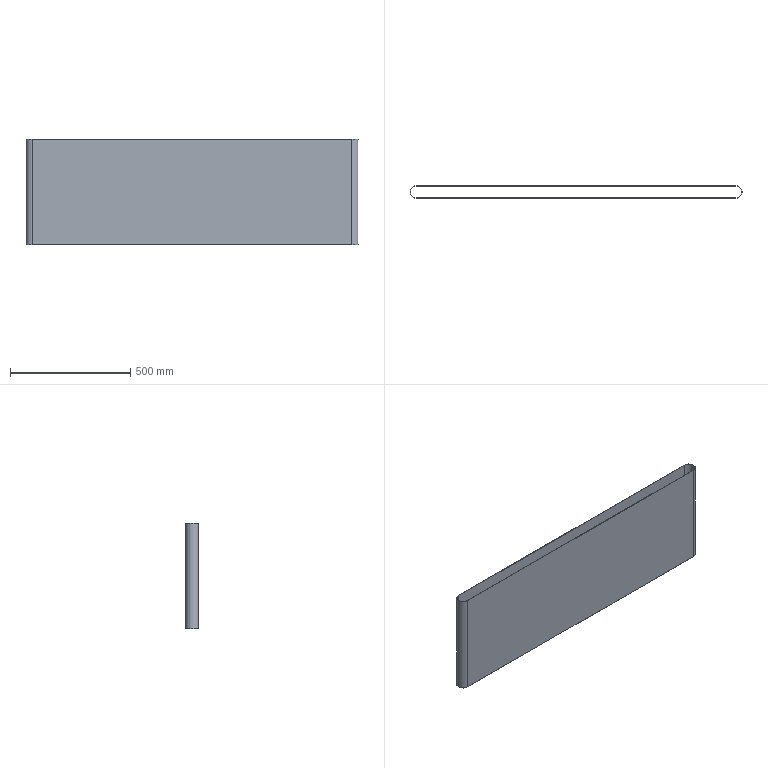Part | STEP file | RUBE 615 | 1 solid | 10 faces | box 1381 x 53.2 x 440 mm | volume 1983947 mm3 | plane 6 | cylinder 4 | commonest cylinder face diameters 50 x2 53.2 x2
STEP:
#1=CARTESIAN_POINT('',(-1248.5,28.6,220.));
#2=VERTEX_POINT('',#1);
#3=CARTESIAN_POINT('',(-1248.5,-24.6,220.));
#4=VERTEX_POINT('',#3);
#5=CARTESIAN_POINT('',(-1248.5,2.,220.));
#6=DIRECTION('',(0.,0.,1.));
#7=DIRECTION('',(1.,0.,0.));
#8=AXIS2_PLACEMENT_3D('',#5,#6,#7);
#9=CIRCLE('',#8,26.6);
#10=EDGE_CURVE('',#2,#4,#9,.T.);
#11=ORIENTED_EDGE('',*,*,#10,.T.);
#12=CARTESIAN_POINT('',(79.5,-24.6,220.));
#13=VERTEX_POINT('',#12);
#14=CARTESIAN_POINT('',(-1248.5,-24.6,220.));
#15=DIRECTION('',(1.,0.,0.));
#16=VECTOR('',#15,1000.);
#17=LINE('',#14,#16);
#18=EDGE_CURVE('',#4,#13,#17,.T.);
#19=ORIENTED_EDGE('',*,*,#18,.T.);
#20=CARTESIAN_POINT('',(79.5,28.6,220.));
#21=VERTEX_POINT('',#20);
#22=CARTESIAN_POINT('',(79.5,2.,220.));
#23=DIRECTION('',(0.,0.,1.));
#24=DIRECTION('',(1.,0.,0.));
#25=AXIS2_PLACEMENT_3D('',#22,#23,#24);
#26=CIRCLE('',#25,26.6);
#27=EDGE_CURVE('',#13,#21,#26,.T.);
#28=ORIENTED_EDGE('',*,*,#27,.T.);
#29=CARTESIAN_POINT('',(-1248.5,28.6,220.));
#30=DIRECTION('',(-1.,0.,0.));
#31=VECTOR('',#30,1000.);
#32=LINE('',#29,#31);
#33=EDGE_CURVE('',#21,#2,#32,.T.);
#34=ORIENTED_EDGE('',*,*,#33,.T.);
#35=EDGE_LOOP('',(#11,#19,#28,#34));
#36=FACE_OUTER_BOUND('',#35,.T.);
#37=CARTESIAN_POINT('',(-1248.5,-23.,220.));
#38=VERTEX_POINT('',#37);
#39=CARTESIAN_POINT('',(79.5,-23.,220.));
#40=VERTEX_POINT('',#39);
#41=CARTESIAN_POINT('',(-1248.5,-23.,220.));
#42=DIRECTION('',(1.,0.,0.));
#43=VECTOR('',#42,1000.);
#44=LINE('',#41,#43);
#45=EDGE_CURVE('',#38,#40,#44,.T.);
#46=ORIENTED_EDGE('',*,*,#45,.F.);
#47=CARTESIAN_POINT('',(-1248.5,27.,220.));
#48=VERTEX_POINT('',#47);
#49=CARTESIAN_POINT('',(-1248.5,2.,220.));
#50=DIRECTION('',(0.,0.,1.));
#51=DIRECTION('',(1.,0.,0.));
#52=AXIS2_PLACEMENT_3D('',#49,#50,#51);
#53=CIRCLE('',#52,25.);
#54=EDGE_CURVE('',#48,#38,#53,.T.);
#55=ORIENTED_EDGE('',*,*,#54,.F.);
#56=CARTESIAN_POINT('',(79.5,27.,220.));
#57=VERTEX_POINT('',#56);
#58=CARTESIAN_POINT('',(-1248.5,27.,220.));
#59=DIRECTION('',(-1.,0.,0.));
#60=VECTOR('',#59,1000.);
#61=LINE('',#58,#60);
#62=EDGE_CURVE('',#57,#48,#61,.T.);
#63=ORIENTED_EDGE('',*,*,#62,.F.);
#64=CARTESIAN_POINT('',(79.5,2.,220.));
#65=DIRECTION('',(0.,0.,1.));
#66=DIRECTION('',(1.,0.,0.));
#67=AXIS2_PLACEMENT_3D('',#64,#65,#66);
#68=CIRCLE('',#67,25.);
#69=EDGE_CURVE('',#40,#57,#68,.T.);
#70=ORIENTED_EDGE('',*,*,#69,.F.);
#71=EDGE_LOOP('',(#46,#55,#63,#70));
#72=FACE_BOUND('',#71,.T.);
#73=CARTESIAN_POINT('',(-1248.5,2.,220.));
#74=DIRECTION('',(0.,0.,1.));
#75=DIRECTION('',(1.,0.,0.));
#76=AXIS2_PLACEMENT_3D('',#73,#74,#75);
#77=PLANE('',#76);
#78=ADVANCED_FACE('',(#36,#72),#77,.T.);
#79=CARTESIAN_POINT('',(-1248.5,28.6,-220.));
#80=VERTEX_POINT('',#79);
#81=CARTESIAN_POINT('',(-1248.5,-24.6,-220.));
#82=VERTEX_POINT('',#81);
#83=CARTESIAN_POINT('',(-1248.5,2.,-220.));
#84=DIRECTION('',(0.,0.,1.));
#85=DIRECTION('',(1.,0.,0.));
#86=AXIS2_PLACEMENT_3D('',#83,#84,#85);
#87=CIRCLE('',#86,26.6);
#88=EDGE_CURVE('',#80,#82,#87,.T.);
#89=ORIENTED_EDGE('',*,*,#88,.F.);
#90=CARTESIAN_POINT('',(79.5,28.6,-220.));
#91=VERTEX_POINT('',#90);
#92=CARTESIAN_POINT('',(-1248.5,28.6,-220.));
#93=DIRECTION('',(-1.,0.,0.));
#94=VECTOR('',#93,1000.);
#95=LINE('',#92,#94);
#96=EDGE_CURVE('',#91,#80,#95,.T.);
#97=ORIENTED_EDGE('',*,*,#96,.F.);
#98=CARTESIAN_POINT('',(79.5,-24.6,-220.));
#99=VERTEX_POINT('',#98);
#100=CARTESIAN_POINT('',(79.5,2.,-220.));
#101=DIRECTION('',(0.,0.,1.));
#102=DIRECTION('',(1.,0.,0.));
#103=AXIS2_PLACEMENT_3D('',#100,#101,#102);
#104=CIRCLE('',#103,26.6);
#105=EDGE_CURVE('',#99,#91,#104,.T.);
#106=ORIENTED_EDGE('',*,*,#105,.F.);
#107=CARTESIAN_POINT('',(-1248.5,-24.6,-220.));
#108=DIRECTION('',(1.,0.,0.));
#109=VECTOR('',#108,1000.);
#110=LINE('',#107,#109);
#111=EDGE_CURVE('',#82,#99,#110,.T.);
#112=ORIENTED_EDGE('',*,*,#111,.F.);
#113=EDGE_LOOP('',(#89,#97,#106,#112));
#114=FACE_OUTER_BOUND('',#113,.T.);
#115=CARTESIAN_POINT('',(-1248.5,27.,-220.));
#116=VERTEX_POINT('',#115);
#117=CARTESIAN_POINT('',(-1248.5,-23.,-220.));
#118=VERTEX_POINT('',#117);
#119=CARTESIAN_POINT('',(-1248.5,2.,-220.));
#120=DIRECTION('',(0.,0.,1.));
#121=DIRECTION('',(1.,0.,0.));
#122=AXIS2_PLACEMENT_3D('',#119,#120,#121);
#123=CIRCLE('',#122,25.);
#124=EDGE_CURVE('',#116,#118,#123,.T.);
#125=ORIENTED_EDGE('',*,*,#124,.T.);
#126=CARTESIAN_POINT('',(79.5,-23.,-220.));
#127=VERTEX_POINT('',#126);
#128=CARTESIAN_POINT('',(-1248.5,-23.,-220.));
#129=DIRECTION('',(1.,0.,0.));
#130=VECTOR('',#129,1000.);
#131=LINE('',#128,#130);
#132=EDGE_CURVE('',#118,#127,#131,.T.);
#133=ORIENTED_EDGE('',*,*,#132,.T.);
#134=CARTESIAN_POINT('',(79.5,27.,-220.));
#135=VERTEX_POINT('',#134);
#136=CARTESIAN_POINT('',(79.5,2.,-220.));
#137=DIRECTION('',(0.,0.,1.));
#138=DIRECTION('',(1.,0.,0.));
#139=AXIS2_PLACEMENT_3D('',#136,#137,#138);
#140=CIRCLE('',#139,25.);
#141=EDGE_CURVE('',#127,#135,#140,.T.);
#142=ORIENTED_EDGE('',*,*,#141,.T.);
#143=CARTESIAN_POINT('',(-1248.5,27.,-220.));
#144=DIRECTION('',(-1.,0.,0.));
#145=VECTOR('',#144,1000.);
#146=LINE('',#143,#145);
#147=EDGE_CURVE('',#135,#116,#146,.T.);
#148=ORIENTED_EDGE('',*,*,#147,.T.);
#149=EDGE_LOOP('',(#125,#133,#142,#148));
#150=FACE_BOUND('',#149,.T.);
#151=CARTESIAN_POINT('',(-1248.5,2.,-220.));
#152=DIRECTION('',(0.,0.,1.));
#153=DIRECTION('',(1.,0.,0.));
#154=AXIS2_PLACEMENT_3D('',#151,#152,#153);
#155=PLANE('',#154);
#156=ADVANCED_FACE('',(#114,#150),#155,.F.);
#157=ORIENTED_EDGE('',*,*,#88,.T.);
#158=CARTESIAN_POINT('',(-1248.5,-24.6,220.));
#159=DIRECTION('',(0.,0.,-1.));
#160=VECTOR('',#159,1000.);
#161=LINE('',#158,#160);
#162=EDGE_CURVE('',#4,#82,#161,.T.);
#163=ORIENTED_EDGE('',*,*,#162,.F.);
#164=ORIENTED_EDGE('',*,*,#10,.F.);
#165=CARTESIAN_POINT('',(-1248.5,28.6,220.));
#166=DIRECTION('',(0.,0.,-1.));
#167=VECTOR('',#166,1000.);
#168=LINE('',#165,#167);
#169=EDGE_CURVE('',#2,#80,#168,.T.);
#170=ORIENTED_EDGE('',*,*,#169,.T.);
#171=EDGE_LOOP('',(#157,#163,#164,#170));
#172=FACE_OUTER_BOUND('',#171,.T.);
#173=CARTESIAN_POINT('',(-1248.5,2.,220.));
#174=DIRECTION('',(0.,0.,-1.));
#175=DIRECTION('',(-1.,0.,0.));
#176=AXIS2_PLACEMENT_3D('',#173,#174,#175);
#177=CYLINDRICAL_SURFACE('',#176,26.6);
#178=ADVANCED_FACE('',(#172),#177,.T.);
#179=ORIENTED_EDGE('',*,*,#111,.T.);
#180=CARTESIAN_POINT('',(79.5,-24.6,220.));
#181=DIRECTION('',(0.,0.,-1.));
#182=VECTOR('',#181,1000.);
#183=LINE('',#180,#182);
#184=EDGE_CURVE('',#13,#99,#183,.T.);
#185=ORIENTED_EDGE('',*,*,#184,.F.);
#186=ORIENTED_EDGE('',*,*,#18,.F.);
#187=ORIENTED_EDGE('',*,*,#162,.T.);
#188=EDGE_LOOP('',(#179,#185,#186,#187));
#189=FACE_OUTER_BOUND('',#188,.T.);
#190=CARTESIAN_POINT('',(-1248.5,-24.6,220.));
#191=DIRECTION('',(0.,1.,0.));
#192=DIRECTION('',(-1.,0.,0.));
#193=AXIS2_PLACEMENT_3D('',#190,#191,#192);
#194=PLANE('',#193);
#195=ADVANCED_FACE('',(#189),#194,.F.);
#196=ORIENTED_EDGE('',*,*,#105,.T.);
#197=CARTESIAN_POINT('',(79.5,28.6,220.));
#198=DIRECTION('',(0.,0.,-1.));
#199=VECTOR('',#198,1000.);
#200=LINE('',#197,#199);
#201=EDGE_CURVE('',#21,#91,#200,.T.);
#202=ORIENTED_EDGE('',*,*,#201,.F.);
#203=ORIENTED_EDGE('',*,*,#27,.F.);
#204=ORIENTED_EDGE('',*,*,#184,.T.);
#205=EDGE_LOOP('',(#196,#202,#203,#204));
#206=FACE_OUTER_BOUND('',#205,.T.);
#207=CARTESIAN_POINT('',(79.5,2.,220.));
#208=DIRECTION('',(0.,0.,-1.));
#209=DIRECTION('',(-1.,0.,0.));
#210=AXIS2_PLACEMENT_3D('',#207,#208,#209);
#211=CYLINDRICAL_SURFACE('',#210,26.6);
#212=ADVANCED_FACE('',(#206),#211,.T.);
#213=ORIENTED_EDGE('',*,*,#96,.T.);
#214=ORIENTED_EDGE('',*,*,#169,.F.);
#215=ORIENTED_EDGE('',*,*,#33,.F.);
#216=ORIENTED_EDGE('',*,*,#201,.T.);
#217=EDGE_LOOP('',(#213,#214,#215,#216));
#218=FACE_OUTER_BOUND('',#217,.T.);
#219=CARTESIAN_POINT('',(-1248.5,28.6,220.));
#220=DIRECTION('',(0.,-1.,0.));
#221=DIRECTION('',(1.,0.,0.));
#222=AXIS2_PLACEMENT_3D('',#219,#220,#221);
#223=PLANE('',#222);
#224=ADVANCED_FACE('',(#218),#223,.F.);
#225=ORIENTED_EDGE('',*,*,#124,.F.);
#226=CARTESIAN_POINT('',(-1248.5,27.,220.));
#227=DIRECTION('',(0.,0.,-1.));
#228=VECTOR('',#227,1000.);
#229=LINE('',#226,#228);
#230=EDGE_CURVE('',#48,#116,#229,.T.);
#231=ORIENTED_EDGE('',*,*,#230,.F.);
#232=ORIENTED_EDGE('',*,*,#54,.T.);
#233=CARTESIAN_POINT('',(-1248.5,-23.,220.));
#234=DIRECTION('',(0.,0.,-1.));
#235=VECTOR('',#234,1000.);
#236=LINE('',#233,#235);
#237=EDGE_CURVE('',#38,#118,#236,.T.);
#238=ORIENTED_EDGE('',*,*,#237,.T.);
#239=EDGE_LOOP('',(#225,#231,#232,#238));
#240=FACE_OUTER_BOUND('',#239,.T.);
#241=CARTESIAN_POINT('',(-1248.5,2.,220.));
#242=DIRECTION('',(0.,0.,-1.));
#243=DIRECTION('',(-1.,0.,0.));
#244=AXIS2_PLACEMENT_3D('',#241,#242,#243);
#245=CYLINDRICAL_SURFACE('',#244,25.);
#246=ADVANCED_FACE('',(#240),#245,.F.);
#247=ORIENTED_EDGE('',*,*,#132,.F.);
#248=ORIENTED_EDGE('',*,*,#237,.F.);
#249=ORIENTED_EDGE('',*,*,#45,.T.);
#250=CARTESIAN_POINT('',(79.5,-23.,220.));
#251=DIRECTION('',(0.,0.,-1.));
#252=VECTOR('',#251,1000.);
#253=LINE('',#250,#252);
#254=EDGE_CURVE('',#40,#127,#253,.T.);
#255=ORIENTED_EDGE('',*,*,#254,.T.);
#256=EDGE_LOOP('',(#247,#248,#249,#255));
#257=FACE_OUTER_BOUND('',#256,.T.);
#258=CARTESIAN_POINT('',(-1248.5,-23.,220.));
#259=DIRECTION('',(0.,1.,0.));
#260=DIRECTION('',(-1.,0.,0.));
#261=AXIS2_PLACEMENT_3D('',#258,#259,#260);
#262=PLANE('',#261);
#263=ADVANCED_FACE('',(#257),#262,.T.);
#264=ORIENTED_EDGE('',*,*,#141,.F.);
#265=ORIENTED_EDGE('',*,*,#254,.F.);
#266=ORIENTED_EDGE('',*,*,#69,.T.);
#267=CARTESIAN_POINT('',(79.5,27.,220.));
#268=DIRECTION('',(0.,0.,-1.));
#269=VECTOR('',#268,1000.);
#270=LINE('',#267,#269);
#271=EDGE_CURVE('',#57,#135,#270,.T.);
#272=ORIENTED_EDGE('',*,*,#271,.T.);
#273=EDGE_LOOP('',(#264,#265,#266,#272));
#274=FACE_OUTER_BOUND('',#273,.T.);
#275=CARTESIAN_POINT('',(79.5,2.,220.));
#276=DIRECTION('',(0.,0.,-1.));
#277=DIRECTION('',(-1.,0.,0.));
#278=AXIS2_PLACEMENT_3D('',#275,#276,#277);
#279=CYLINDRICAL_SURFACE('',#278,25.);
#280=ADVANCED_FACE('',(#274),#279,.F.);
#281=ORIENTED_EDGE('',*,*,#147,.F.);
#282=ORIENTED_EDGE('',*,*,#271,.F.);
#283=ORIENTED_EDGE('',*,*,#62,.T.);
#284=ORIENTED_EDGE('',*,*,#230,.T.);
#285=EDGE_LOOP('',(#281,#282,#283,#284));
#286=FACE_OUTER_BOUND('',#285,.T.);
#287=CARTESIAN_POINT('',(-1248.5,27.,220.));
#288=DIRECTION('',(0.,-1.,0.));
#289=DIRECTION('',(1.,0.,0.));
#290=AXIS2_PLACEMENT_3D('',#287,#288,#289);
#291=PLANE('',#290);
#292=ADVANCED_FACE('',(#286),#291,.T.);
#293=CLOSED_SHELL('',(#78,#156,#178,#195,#212,#224,#246,#263,#280,#292));
#294=MANIFOLD_SOLID_BREP('',#293);
#295=CARTESIAN_POINT('',(0.,0.,0.));
#296=DIRECTION('',(0.,0.,1.));
#297=DIRECTION('',(1.,0.,0.));
#298=AXIS2_PLACEMENT_3D('',#295,#296,#297);
#299=(LENGTH_UNIT()NAMED_UNIT(*)SI_UNIT(.MILLI.,.METRE.));
#300=UNCERTAINTY_MEASURE_WITH_UNIT(LENGTH_MEASURE(0.00001),#299,'','');
#301=(NAMED_UNIT(*)PLANE_ANGLE_UNIT()SI_UNIT($,.RADIAN.));
#302=(NAMED_UNIT(*)SI_UNIT($,.STERADIAN.)SOLID_ANGLE_UNIT());
#303=(GEOMETRIC_REPRESENTATION_CONTEXT(3)GLOBAL_UNCERTAINTY_ASSIGNED_CONTEXT((#300))GLOBAL_UNIT_ASSIGNED_CONTEXT((#299,#301,#302))REPRESENTATION_CONTEXT('',''));
#304=ADVANCED_BREP_SHAPE_REPRESENTATION('',(#294,#298),#303);